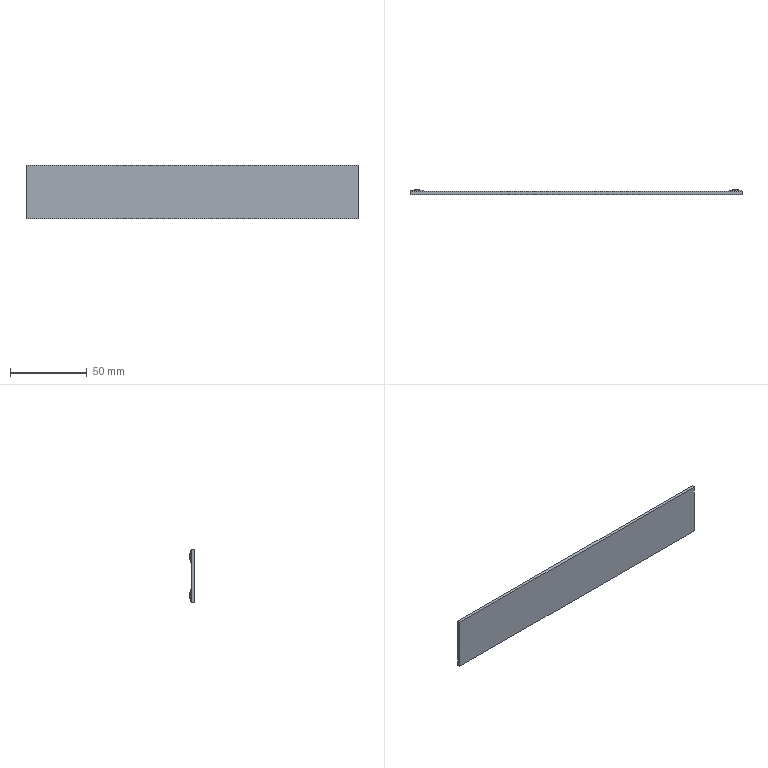Part | STEP file | QA-LX2005C_B1_200_c | 1 solid | 34 faces | box 216 x 3.2 x 35 mm | volume 15277 mm3 | cylinder 16 | plane 10 | cone 8 | commonest cylinder face diameters 3.8 x8 8 x8